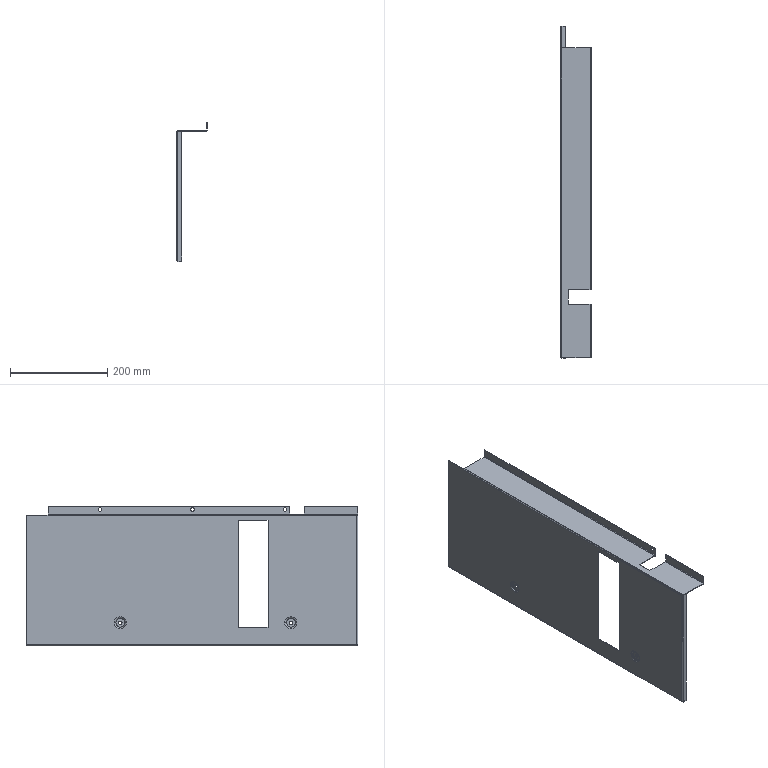Part | STEP file | 1 solid | 98 faces | box 62 x 681 x 286 mm | volume 269371 mm3 | plane 54 | cylinder 28 | torus 16 | commonest cylinder face diameters 7 x10 2 x5 4.4 x5 20 x4 22.4 x4